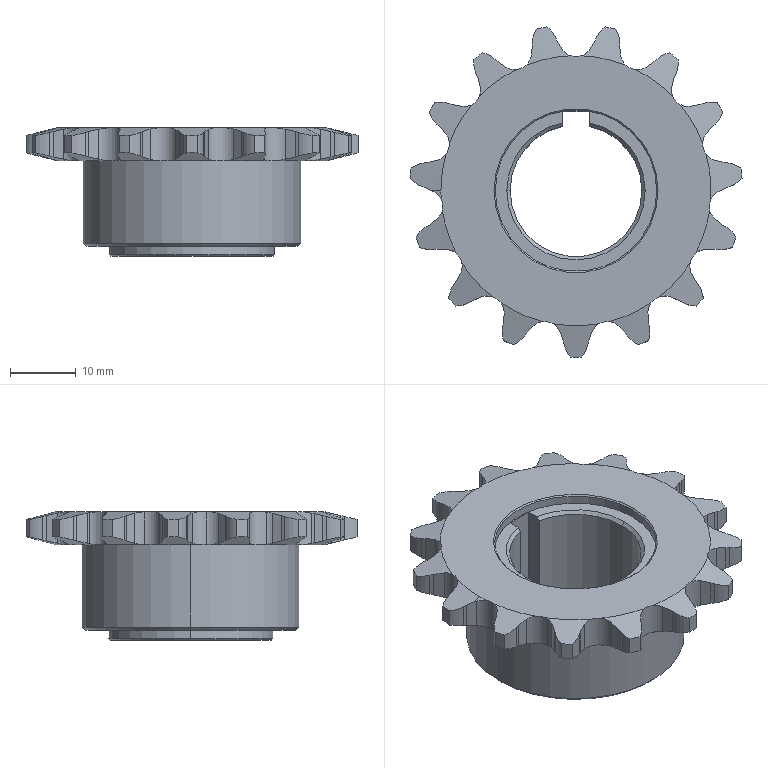Part | STEP file | BZJ-LSX-RGX 主动链轮06B-15齿_内Holeφ20_J | 1 solid | 188 faces | box 50.395 x 50.132 x 19.5 mm | volume 13040 mm3 | cylinder 106 | cone 44 | plane 38 | commonest cylinder face diameters 8.515 x32 13.236 x31 5.108 x19 50.527 x15 20 x3 24.5 x2